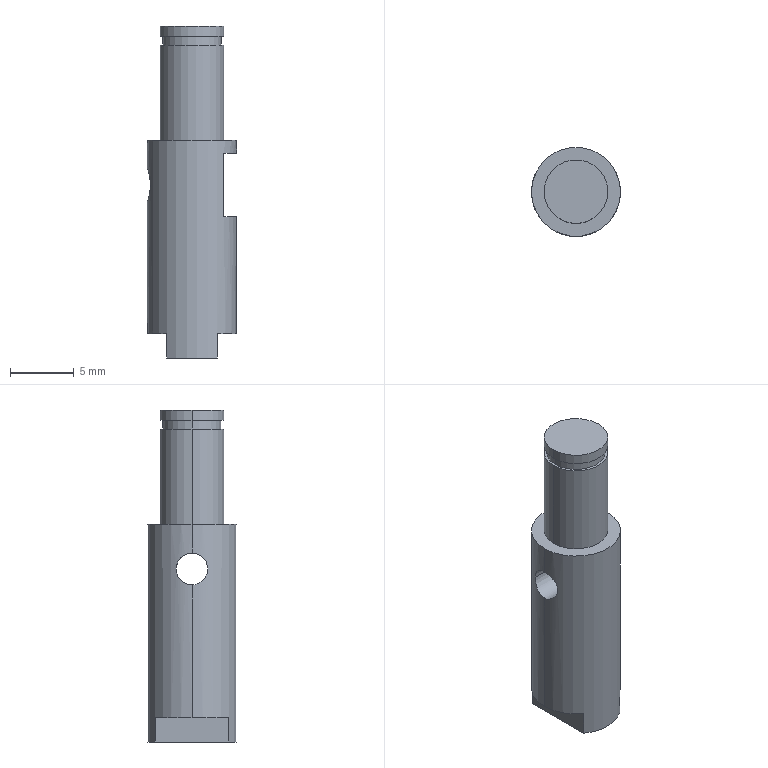Part | NX | 1 solid | 30 faces | box 7 x 7 x 26.1 mm | volume 718.496 mm3 | plane 12 | cylinder 12 | cone 6 | commonest cylinder face diameters 2.5 x4 5 x4 4.6 x2 7 x2
STEP:
#1=CARTESIAN_POINT('',(-2.5,0.,9.));
#2=VERTEX_POINT('',#1);
#3=CARTESIAN_POINT('',(2.5,0.,9.));
#4=VERTEX_POINT('',#3);
#5=CARTESIAN_POINT('',(0.,0.,9.));
#6=DIRECTION('',(0.,0.,-1.));
#7=DIRECTION('',(1.,0.,0.));
#8=AXIS2_PLACEMENT_3D('',#5,#6,#7);
#9=CIRCLE('',#8,2.5);
#10=EDGE_CURVE('',#2,#4,#9,.T.);
#11=ORIENTED_EDGE('',*,*,#10,.F.);
#12=CARTESIAN_POINT('',(0.,0.,9.));
#13=DIRECTION('',(0.,0.,-1.));
#14=DIRECTION('',(1.,0.,0.));
#15=AXIS2_PLACEMENT_3D('',#12,#13,#14);
#16=CIRCLE('',#15,2.5);
#17=EDGE_CURVE('',#4,#2,#16,.T.);
#18=ORIENTED_EDGE('',*,*,#17,.F.);
#19=EDGE_LOOP('',(#11,#18));
#20=FACE_BOUND('',#19,.T.);
#21=CARTESIAN_POINT('',(0.,0.,9.));
#22=DIRECTION('',(0.,0.,1.));
#23=DIRECTION('',(1.,0.,0.));
#24=AXIS2_PLACEMENT_3D('',#21,#22,#23);
#25=PLANE('',#24);
#26=ADVANCED_FACE('',(#20),#25,.T.);
#27=ORIENTED_EDGE('',*,*,#10,.T.);
#28=CARTESIAN_POINT('',(2.5,0.,8.2));
#29=VERTEX_POINT('',#28);
#30=CARTESIAN_POINT('',(2.5,0.,0.));
#31=DIRECTION('',(0.,0.,1.));
#32=VECTOR('',#31,1000.);
#33=LINE('',#30,#32);
#34=EDGE_CURVE('',#29,#4,#33,.T.);
#35=ORIENTED_EDGE('',*,*,#34,.F.);
#36=CARTESIAN_POINT('',(-2.5,0.,8.2));
#37=VERTEX_POINT('',#36);
#38=CARTESIAN_POINT('',(0.,0.,8.2));
#39=DIRECTION('',(0.,0.,1.));
#40=DIRECTION('',(-1.,0.,0.));
#41=AXIS2_PLACEMENT_3D('',#38,#39,#40);
#42=CIRCLE('',#41,2.5);
#43=EDGE_CURVE('',#29,#37,#42,.T.);
#44=ORIENTED_EDGE('',*,*,#43,.T.);
#45=CARTESIAN_POINT('',(-2.5,0.,0.));
#46=DIRECTION('',(0.,0.,1.));
#47=VECTOR('',#46,1000.);
#48=LINE('',#45,#47);
#49=EDGE_CURVE('',#37,#2,#48,.T.);
#50=ORIENTED_EDGE('',*,*,#49,.T.);
#51=EDGE_LOOP('',(#27,#35,#44,#50));
#52=FACE_BOUND('',#51,.T.);
#53=CARTESIAN_POINT('',(0.,0.,0.));
#54=DIRECTION('',(0.,0.,1.));
#55=DIRECTION('',(1.,0.,0.));
#56=AXIS2_PLACEMENT_3D('',#53,#54,#55);
#57=CYLINDRICAL_SURFACE('',#56,2.5);
#58=ADVANCED_FACE('',(#52),#57,.T.);
#59=ORIENTED_EDGE('',*,*,#43,.F.);
#60=CARTESIAN_POINT('',(0.,0.,8.2));
#61=DIRECTION('',(0.,0.,1.));
#62=DIRECTION('',(-1.,0.,0.));
#63=AXIS2_PLACEMENT_3D('',#60,#61,#62);
#64=CIRCLE('',#63,2.5);
#65=EDGE_CURVE('',#37,#29,#64,.T.);
#66=ORIENTED_EDGE('',*,*,#65,.F.);
#67=EDGE_LOOP('',(#59,#66));
#68=FACE_BOUND('',#67,.T.);
#69=CARTESIAN_POINT('',(2.3,0.,8.2));
#70=VERTEX_POINT('',#69);
#71=CARTESIAN_POINT('',(-2.3,0.,8.2));
#72=VERTEX_POINT('',#71);
#73=CARTESIAN_POINT('',(0.,0.,8.2));
#74=DIRECTION('',(0.,0.,-1.));
#75=DIRECTION('',(1.,0.,0.));
#76=AXIS2_PLACEMENT_3D('',#73,#74,#75);
#77=CIRCLE('',#76,2.3);
#78=EDGE_CURVE('',#70,#72,#77,.T.);
#79=ORIENTED_EDGE('',*,*,#78,.F.);
#80=CARTESIAN_POINT('',(0.,0.,8.2));
#81=DIRECTION('',(0.,0.,-1.));
#82=DIRECTION('',(1.,0.,0.));
#83=AXIS2_PLACEMENT_3D('',#80,#81,#82);
#84=CIRCLE('',#83,2.3);
#85=EDGE_CURVE('',#72,#70,#84,.T.);
#86=ORIENTED_EDGE('',*,*,#85,.F.);
#87=EDGE_LOOP('',(#79,#86));
#88=FACE_BOUND('',#87,.T.);
#89=CARTESIAN_POINT('',(0.,0.,8.2));
#90=DIRECTION('',(0.,0.,-1.));
#91=DIRECTION('',(0.,-1.,0.));
#92=AXIS2_PLACEMENT_3D('',#89,#90,#91);
#93=PLANE('',#92);
#94=ADVANCED_FACE('',(#68,#88),#93,.T.);
#95=CARTESIAN_POINT('',(-2.,2.872,-17.1));
#96=VERTEX_POINT('',#95);
#97=CARTESIAN_POINT('',(2.,2.872,-17.1));
#98=VERTEX_POINT('',#97);
#99=CARTESIAN_POINT('',(0.,0.,-17.1));
#100=DIRECTION('',(0.,0.,-1.));
#101=DIRECTION('',(-1.,0.,0.));
#102=AXIS2_PLACEMENT_3D('',#99,#100,#101);
#103=CIRCLE('',#102,3.5);
#104=EDGE_CURVE('',#96,#98,#103,.T.);
#105=ORIENTED_EDGE('',*,*,#104,.T.);
#106=CARTESIAN_POINT('',(2.,-2.872,-17.1));
#107=VERTEX_POINT('',#106);
#108=CARTESIAN_POINT('',(2.,0.,-17.1));
#109=DIRECTION('',(0.,-1.,0.));
#110=VECTOR('',#109,1000.);
#111=LINE('',#108,#110);
#112=EDGE_CURVE('',#98,#107,#111,.T.);
#113=ORIENTED_EDGE('',*,*,#112,.T.);
#114=CARTESIAN_POINT('',(-2.,-2.872,-17.1));
#115=VERTEX_POINT('',#114);
#116=CARTESIAN_POINT('',(0.,0.,-17.1));
#117=DIRECTION('',(0.,0.,-1.));
#118=DIRECTION('',(-1.,0.,0.));
#119=AXIS2_PLACEMENT_3D('',#116,#117,#118);
#120=CIRCLE('',#119,3.5);
#121=EDGE_CURVE('',#107,#115,#120,.T.);
#122=ORIENTED_EDGE('',*,*,#121,.T.);
#123=CARTESIAN_POINT('',(-2.,0.,-17.1));
#124=DIRECTION('',(0.,-1.,0.));
#125=VECTOR('',#124,1000.);
#126=LINE('',#123,#125);
#127=EDGE_CURVE('',#96,#115,#126,.T.);
#128=ORIENTED_EDGE('',*,*,#127,.F.);
#129=EDGE_LOOP('',(#105,#113,#122,#128));
#130=FACE_BOUND('',#129,.T.);
#131=CARTESIAN_POINT('',(1.7,0.,-17.1));
#132=VERTEX_POINT('',#131);
#133=CARTESIAN_POINT('',(-1.7,0.,-17.1));
#134=VERTEX_POINT('',#133);
#135=CARTESIAN_POINT('',(0.,0.,-17.1));
#136=DIRECTION('',(0.,0.,-1.));
#137=DIRECTION('',(-1.,0.,0.));
#138=AXIS2_PLACEMENT_3D('',#135,#136,#137);
#139=CIRCLE('',#138,1.7);
#140=EDGE_CURVE('',#132,#134,#139,.T.);
#141=ORIENTED_EDGE('',*,*,#140,.F.);
#142=CARTESIAN_POINT('',(0.,0.,-17.1));
#143=DIRECTION('',(0.,0.,-1.));
#144=DIRECTION('',(-1.,0.,0.));
#145=AXIS2_PLACEMENT_3D('',#142,#143,#144);
#146=CIRCLE('',#145,1.7);
#147=EDGE_CURVE('',#134,#132,#146,.T.);
#148=ORIENTED_EDGE('',*,*,#147,.F.);
#149=EDGE_LOOP('',(#141,#148));
#150=FACE_BOUND('',#149,.T.);
#151=CARTESIAN_POINT('',(0.,0.,-17.1));
#152=DIRECTION('',(0.,0.,-1.));
#153=DIRECTION('',(0.,-1.,0.));
#154=AXIS2_PLACEMENT_3D('',#151,#152,#153);
#155=PLANE('',#154);
#156=ADVANCED_FACE('',(#130,#150),#155,.T.);
#157=ORIENTED_EDGE('',*,*,#78,.T.);
#158=CARTESIAN_POINT('',(-2.3,0.,7.5));
#159=VERTEX_POINT('',#158);
#160=CARTESIAN_POINT('',(-2.3,0.,8.235));
#161=DIRECTION('',(0.,0.,-1.));
#162=VECTOR('',#161,1000.);
#163=LINE('',#160,#162);
#164=EDGE_CURVE('',#159,#72,#163,.F.);
#165=ORIENTED_EDGE('',*,*,#164,.F.);
#166=CARTESIAN_POINT('',(2.3,0.,7.5));
#167=VERTEX_POINT('',#166);
#168=CARTESIAN_POINT('',(0.,0.,7.5));
#169=DIRECTION('',(0.,0.,1.));
#170=DIRECTION('',(1.,0.,0.));
#171=AXIS2_PLACEMENT_3D('',#168,#169,#170);
#172=CIRCLE('',#171,2.3);
#173=EDGE_CURVE('',#159,#167,#172,.T.);
#174=ORIENTED_EDGE('',*,*,#173,.T.);
#175=CARTESIAN_POINT('',(2.3,0.,8.235));
#176=DIRECTION('',(0.,0.,-1.));
#177=VECTOR('',#176,1000.);
#178=LINE('',#175,#177);
#179=EDGE_CURVE('',#167,#70,#178,.F.);
#180=ORIENTED_EDGE('',*,*,#179,.T.);
#181=EDGE_LOOP('',(#157,#165,#174,#180));
#182=FACE_BOUND('',#181,.T.);
#183=CARTESIAN_POINT('',(0.,0.,8.235));
#184=DIRECTION('',(0.,0.,-1.));
#185=DIRECTION('',(-1.,0.,0.));
#186=AXIS2_PLACEMENT_3D('',#183,#184,#185);
#187=CYLINDRICAL_SURFACE('',#186,2.3);
#188=ADVANCED_FACE('',(#182),#187,.T.);
#189=CARTESIAN_POINT('',(-3.269,1.25,-3.5));
#190=VERTEX_POINT('',#189);
#191=CARTESIAN_POINT('',(-3.5,0.,-2.25));
#192=VERTEX_POINT('',#191);
#193=CARTESIAN_POINT('',(-3.5,0.,-2.25));
#194=CARTESIAN_POINT('',(-3.5,0.1562,-2.25));
#195=CARTESIAN_POINT('',(-3.476,0.4429,-2.317));
#196=CARTESIAN_POINT('',(-3.44,0.6524,-2.427));
#197=CARTESIAN_POINT('',(-3.387,0.8925,-2.603));
#198=CARTESIAN_POINT('',(-3.33,1.082,-2.861));
#199=CARTESIAN_POINT('',(-3.296,1.178,-3.049));
#200=CARTESIAN_POINT('',(-3.269,1.25,-3.345));
#201=CARTESIAN_POINT('',(-3.269,1.25,-3.5));
#202=B_SPLINE_CURVE_WITH_KNOTS('',3,(#193,#194,#195,#196,#197,#198,#199,#200,#201),.UNSPECIFIED.,.F.,.F.,(4,1,1,1,1,1,4),(0.,0.25,0.375,0.5,0.625,0.75,1.),.UNSPECIFIED.);
#203=EDGE_CURVE('',#190,#192,#202,.F.);
#204=ORIENTED_EDGE('',*,*,#203,.F.);
#205=CARTESIAN_POINT('',(2.24,1.25,-3.5));
#206=VERTEX_POINT('',#205);
#207=CARTESIAN_POINT('',(2.5,1.25,-3.5));
#208=DIRECTION('',(1.,0.,0.));
#209=VECTOR('',#208,1000.);
#210=LINE('',#207,#209);
#211=EDGE_CURVE('',#190,#206,#210,.T.);
#212=ORIENTED_EDGE('',*,*,#211,.T.);
#213=CARTESIAN_POINT('',(2.24,-1.25,-3.5));
#214=VERTEX_POINT('',#213);
#215=CARTESIAN_POINT('',(2.24,0.,-3.5));
#216=DIRECTION('',(1.,0.,0.));
#217=DIRECTION('',(0.,-1.,0.));
#218=AXIS2_PLACEMENT_3D('',#215,#216,#217);
#219=CIRCLE('',#218,1.25);
#220=EDGE_CURVE('',#206,#214,#219,.T.);
#221=ORIENTED_EDGE('',*,*,#220,.T.);
#222=CARTESIAN_POINT('',(-3.269,-1.25,-3.5));
#223=VERTEX_POINT('',#222);
#224=CARTESIAN_POINT('',(2.5,-1.25,-3.5));
#225=DIRECTION('',(1.,0.,0.));
#226=VECTOR('',#225,1000.);
#227=LINE('',#224,#226);
#228=EDGE_CURVE('',#223,#214,#227,.T.);
#229=ORIENTED_EDGE('',*,*,#228,.F.);
#230=CARTESIAN_POINT('',(-3.269,-1.25,-3.5));
#231=CARTESIAN_POINT('',(-3.269,-1.25,-3.345));
#232=CARTESIAN_POINT('',(-3.296,-1.178,-3.049));
#233=CARTESIAN_POINT('',(-3.33,-1.082,-2.86));
#234=CARTESIAN_POINT('',(-3.387,-0.8925,-2.603));
#235=CARTESIAN_POINT('',(-3.44,-0.6525,-2.427));
#236=CARTESIAN_POINT('',(-3.476,-0.4428,-2.317));
#237=CARTESIAN_POINT('',(-3.5,-0.1562,-2.25));
#238=CARTESIAN_POINT('',(-3.5,0.,-2.25));
#239=B_SPLINE_CURVE_WITH_KNOTS('',3,(#230,#231,#232,#233,#234,#235,#236,#237,#238),.UNSPECIFIED.,.F.,.F.,(4,1,1,1,1,1,4),(0.,0.25,0.375,0.5,0.625,0.75,1.),.UNSPECIFIED.);
#240=EDGE_CURVE('',#192,#223,#239,.F.);
#241=ORIENTED_EDGE('',*,*,#240,.F.);
#242=EDGE_LOOP('',(#204,#212,#221,#229,#241));
#243=FACE_BOUND('',#242,.T.);
#244=CARTESIAN_POINT('',(2.5,0.,-3.5));
#245=DIRECTION('',(1.,0.,0.));
#246=DIRECTION('',(0.,-1.,0.));
#247=AXIS2_PLACEMENT_3D('',#244,#245,#246);
#248=CYLINDRICAL_SURFACE('',#247,1.25);
#249=ADVANCED_FACE('',(#243),#248,.F.);
#250=CARTESIAN_POINT('',(2.5,0.,7.5));
#251=VERTEX_POINT('',#250);
#252=CARTESIAN_POINT('',(-2.5,0.,7.5));
#253=VERTEX_POINT('',#252);
#254=CARTESIAN_POINT('',(0.,0.,7.5));
#255=DIRECTION('',(0.,0.,-1.));
#256=DIRECTION('',(1.,0.,0.));
#257=AXIS2_PLACEMENT_3D('',#254,#255,#256);
#258=CIRCLE('',#257,2.5);
#259=EDGE_CURVE('',#251,#253,#258,.T.);
#260=ORIENTED_EDGE('',*,*,#259,.F.);
#261=CARTESIAN_POINT('',(0.,0.,7.5));
#262=DIRECTION('',(0.,0.,-1.));
#263=DIRECTION('',(1.,0.,0.));
#264=AXIS2_PLACEMENT_3D('',#261,#262,#263);
#265=CIRCLE('',#264,2.5);
#266=EDGE_CURVE('',#253,#251,#265,.T.);
#267=ORIENTED_EDGE('',*,*,#266,.F.);
#268=EDGE_LOOP('',(#260,#267));
#269=FACE_BOUND('',#268,.T.);
#270=ORIENTED_EDGE('',*,*,#173,.F.);
#271=CARTESIAN_POINT('',(0.,0.,7.5));
#272=DIRECTION('',(0.,0.,1.));
#273=DIRECTION('',(1.,0.,0.));
#274=AXIS2_PLACEMENT_3D('',#271,#272,#273);
#275=CIRCLE('',#274,2.3);
#276=EDGE_CURVE('',#167,#159,#275,.T.);
#277=ORIENTED_EDGE('',*,*,#276,.F.);
#278=EDGE_LOOP('',(#270,#277));
#279=FACE_BOUND('',#278,.T.);
#280=CARTESIAN_POINT('',(0.,0.,7.5));
#281=DIRECTION('',(0.,0.,-1.));
#282=DIRECTION('',(0.,-1.,0.));
#283=AXIS2_PLACEMENT_3D('',#280,#281,#282);
#284=PLANE('',#283);
#285=ADVANCED_FACE('',(#269,#279),#284,.F.);
#286=ORIENTED_EDGE('',*,*,#259,.T.);
#287=CARTESIAN_POINT('',(-2.5,0.,0.));
#288=VERTEX_POINT('',#287);
#289=CARTESIAN_POINT('',(-2.5,0.,0.));
#290=DIRECTION('',(0.,0.,1.));
#291=VECTOR('',#290,1000.);
#292=LINE('',#289,#291);
#293=EDGE_CURVE('',#253,#288,#292,.F.);
#294=ORIENTED_EDGE('',*,*,#293,.T.);
#295=CARTESIAN_POINT('',(2.5,0.,0.));
#296=VERTEX_POINT('',#295);
#297=CARTESIAN_POINT('',(0.,0.,0.));
#298=DIRECTION('',(0.,0.,1.));
#299=DIRECTION('',(1.,0.,0.));
#300=AXIS2_PLACEMENT_3D('',#297,#298,#299);
#301=CIRCLE('',#300,2.5);
#302=EDGE_CURVE('',#288,#296,#301,.T.);
#303=ORIENTED_EDGE('',*,*,#302,.T.);
#304=CARTESIAN_POINT('',(2.5,0.,0.));
#305=DIRECTION('',(0.,0.,1.));
#306=VECTOR('',#305,1000.);
#307=LINE('',#304,#306);
#308=EDGE_CURVE('',#251,#296,#307,.F.);
#309=ORIENTED_EDGE('',*,*,#308,.F.);
#310=EDGE_LOOP('',(#286,#294,#303,#309));
#311=FACE_BOUND('',#310,.T.);
#312=CARTESIAN_POINT('',(0.,0.,0.));
#313=DIRECTION('',(0.,0.,1.));
#314=DIRECTION('',(1.,0.,0.));
#315=AXIS2_PLACEMENT_3D('',#312,#313,#314);
#316=CYLINDRICAL_SURFACE('',#315,2.5);
#317=ADVANCED_FACE('',(#311),#316,.T.);
#318=CARTESIAN_POINT('',(2.24,0.,-3.5));
#319=DIRECTION('',(1.,0.,0.));
#320=DIRECTION('',(0.,-1.,0.));
#321=AXIS2_PLACEMENT_3D('',#318,#319,#320);
#322=CIRCLE('',#321,1.25);
#323=EDGE_CURVE('',#214,#206,#322,.T.);
#324=ORIENTED_EDGE('',*,*,#323,.F.);
#325=CARTESIAN_POINT('',(2.5,-1.7,-3.5));
#326=VERTEX_POINT('',#325);
#327=CARTESIAN_POINT('',(2.24,-1.25,-3.5));
#328=DIRECTION('',(0.5,-0.866,0.));
#329=VECTOR('',#328,1000.);
#330=LINE('',#327,#329);
#331=EDGE_CURVE('',#326,#214,#330,.F.);
#332=ORIENTED_EDGE('',*,*,#331,.F.);
#333=CARTESIAN_POINT('',(2.5,1.7,-3.5));
#334=VERTEX_POINT('',#333);
#335=CARTESIAN_POINT('',(2.5,0.,-3.5));
#336=DIRECTION('',(1.,0.,0.));
#337=DIRECTION('',(0.,-1.,0.));
#338=AXIS2_PLACEMENT_3D('',#335,#336,#337);
#339=CIRCLE('',#338,1.7);
#340=EDGE_CURVE('',#326,#334,#339,.T.);
#341=ORIENTED_EDGE('',*,*,#340,.T.);
#342=CARTESIAN_POINT('',(2.24,1.25,-3.5));
#343=DIRECTION('',(0.5,0.866,0.));
#344=VECTOR('',#343,1000.);
#345=LINE('',#342,#344);
#346=EDGE_CURVE('',#334,#206,#345,.F.);
#347=ORIENTED_EDGE('',*,*,#346,.T.);
#348=EDGE_LOOP('',(#324,#332,#341,#347));
#349=FACE_BOUND('',#348,.T.);
#350=CARTESIAN_POINT('',(2.24,0.,-3.5));
#351=DIRECTION('',(1.,0.,0.));
#352=DIRECTION('',(0.,-1.,0.));
#353=AXIS2_PLACEMENT_3D('',#350,#351,#352);
#354=CONICAL_SURFACE('',#353,1.25,1.047);
#355=ADVANCED_FACE('',(#349),#354,.F.);
#356=CARTESIAN_POINT('',(2.5,2.449,-1.));
#357=VERTEX_POINT('',#356);
#358=CARTESIAN_POINT('',(2.5,2.449,-6.));
#359=VERTEX_POINT('',#358);
#360=CARTESIAN_POINT('',(2.5,2.449,0.));
#361=DIRECTION('',(0.,0.,-1.));
#362=VECTOR('',#361,1000.);
#363=LINE('',#360,#362);
#364=EDGE_CURVE('',#357,#359,#363,.T.);
#365=ORIENTED_EDGE('',*,*,#364,.F.);
#366=CARTESIAN_POINT('',(2.5,-2.449,-1.));
#367=VERTEX_POINT('',#366);
#368=CARTESIAN_POINT('',(2.5,0.,-1.));
#369=DIRECTION('',(0.,-1.,0.));
#370=VECTOR('',#369,1000.);
#371=LINE('',#368,#370);
#372=EDGE_CURVE('',#357,#367,#371,.T.);
#373=ORIENTED_EDGE('',*,*,#372,.T.);
#374=CARTESIAN_POINT('',(2.5,-2.449,-6.));
#375=VERTEX_POINT('',#374);
#376=CARTESIAN_POINT('',(2.5,-2.449,0.));
#377=DIRECTION('',(0.,0.,-1.));
#378=VECTOR('',#377,1000.);
#379=LINE('',#376,#378);
#380=EDGE_CURVE('',#367,#375,#379,.T.);
#381=ORIENTED_EDGE('',*,*,#380,.T.);
#382=CARTESIAN_POINT('',(2.5,0.,-6.));
#383=DIRECTION('',(0.,1.,0.));
#384=VECTOR('',#383,1000.);
#385=LINE('',#382,#384);
#386=EDGE_CURVE('',#375,#359,#385,.T.);
#387=ORIENTED_EDGE('',*,*,#386,.T.);
#388=EDGE_LOOP('',(#365,#373,#381,#387));
#389=FACE_BOUND('',#388,.T.);
#390=ORIENTED_EDGE('',*,*,#340,.F.);
#391=CARTESIAN_POINT('',(2.5,0.,-3.5));
#392=DIRECTION('',(1.,0.,0.));
#393=DIRECTION('',(0.,-1.,0.));
#394=AXIS2_PLACEMENT_3D('',#391,#392,#393);
#395=CIRCLE('',#394,1.7);
#396=EDGE_CURVE('',#334,#326,#395,.T.);
#397=ORIENTED_EDGE('',*,*,#396,.F.);
#398=EDGE_LOOP('',(#390,#397));
#399=FACE_BOUND('',#398,.T.);
#400=CARTESIAN_POINT('',(2.5,3.5,-6.));
#401=DIRECTION('',(-1.,0.,0.));
#402=DIRECTION('',(0.,0.,1.));
#403=AXIS2_PLACEMENT_3D('',#400,#401,#402);
#404=PLANE('',#403);
#405=ADVANCED_FACE('',(#389,#399),#404,.F.);
#406=CARTESIAN_POINT('',(3.5,0.,-15.2));
#407=VERTEX_POINT('',#406);
#408=CARTESIAN_POINT('',(2.,-2.872,-15.2));
#409=VERTEX_POINT('',#408);
#410=CARTESIAN_POINT('',(0.,0.,-15.2));
#411=DIRECTION('',(0.,0.,-1.));
#412=DIRECTION('',(-1.,0.,0.));
#413=AXIS2_PLACEMENT_3D('',#410,#411,#412);
#414=CIRCLE('',#413,3.5);
#415=EDGE_CURVE('',#407,#409,#414,.T.);
#416=ORIENTED_EDGE('',*,*,#415,.F.);
#417=CARTESIAN_POINT('',(3.5,0.,-6.));
#418=VERTEX_POINT('',#417);
#419=CARTESIAN_POINT('',(3.5,0.,0.));
#420=DIRECTION('',(0.,0.,-1.));
#421=VECTOR('',#420,1000.);
#422=LINE('',#419,#421);
#423=EDGE_CURVE('',#418,#407,#422,.T.);
#424=ORIENTED_EDGE('',*,*,#423,.F.);
#425=CARTESIAN_POINT('',(0.,0.,-6.));
#426=DIRECTION('',(0.,0.,-1.));
#427=DIRECTION('',(-1.,0.,0.));
#428=AXIS2_PLACEMENT_3D('',#425,#426,#427);
#429=CIRCLE('',#428,3.5);
#430=EDGE_CURVE('',#418,#375,#429,.T.);
#431=ORIENTED_EDGE('',*,*,#430,.T.);
#432=ORIENTED_EDGE('',*,*,#380,.F.);
#433=CARTESIAN_POINT('',(3.5,0.,-1.));
#434=VERTEX_POINT('',#433);
#435=CARTESIAN_POINT('',(0.,0.,-1.));
#436=DIRECTION('',(0.,0.,-1.));
#437=DIRECTION('',(-1.,0.,0.));
#438=AXIS2_PLACEMENT_3D('',#435,#436,#437);
#439=CIRCLE('',#438,3.5);
#440=EDGE_CURVE('',#434,#367,#439,.T.);
#441=ORIENTED_EDGE('',*,*,#440,.F.);
#442=CARTESIAN_POINT('',(3.5,0.,0.));
#443=VERTEX_POINT('',#442);
#444=CARTESIAN_POINT('',(3.5,0.,0.));
#445=DIRECTION('',(0.,0.,-1.));
#446=VECTOR('',#445,1000.);
#447=LINE('',#444,#446);
#448=EDGE_CURVE('',#434,#443,#447,.F.);
#449=ORIENTED_EDGE('',*,*,#448,.T.);
#450=CARTESIAN_POINT('',(-3.5,0.,0.));
#451=VERTEX_POINT('',#450);
#452=CARTESIAN_POINT('',(0.,0.,0.));
#453=DIRECTION('',(0.,0.,-1.));
#454=DIRECTION('',(-1.,0.,0.));
#455=AXIS2_PLACEMENT_3D('',#452,#453,#454);
#456=CIRCLE('',#455,3.5);
#457=EDGE_CURVE('',#443,#451,#456,.T.);
#458=ORIENTED_EDGE('',*,*,#457,.T.);
#459=CARTESIAN_POINT('',(-3.5,0.,0.));
#460=DIRECTION('',(0.,0.,-1.));
#461=VECTOR('',#460,1000.);
#462=LINE('',#459,#461);
#463=EDGE_CURVE('',#192,#451,#462,.F.);
#464=ORIENTED_EDGE('',*,*,#463,.F.);
#465=ORIENTED_EDGE('',*,*,#240,.T.);
#466=CARTESIAN_POINT('',(-3.5,0.,-4.75));
#467=VERTEX_POINT('',#466);
#468=CARTESIAN_POINT('',(-3.269,-1.25,-3.5));
#469=CARTESIAN_POINT('',(-3.269,-1.249,-4.165));
#470=CARTESIAN_POINT('',(-3.5,-0.6651,-4.75));
#471=CARTESIAN_POINT('',(-3.5,0.,-4.75));
#472=B_SPLINE_CURVE_WITH_KNOTS('',3,(#468,#469,#470,#471),.UNSPECIFIED.,.F.,.F.,(4,4),(0.,1.),.UNSPECIFIED.);
#473=EDGE_CURVE('',#223,#467,#472,.T.);
#474=ORIENTED_EDGE('',*,*,#473,.T.);
#475=CARTESIAN_POINT('',(-3.5,0.,-15.2));
#476=VERTEX_POINT('',#475);
#477=CARTESIAN_POINT('',(-3.5,0.,0.));
#478=DIRECTION('',(0.,0.,-1.));
#479=VECTOR('',#478,1000.);
#480=LINE('',#477,#479);
#481=EDGE_CURVE('',#467,#476,#480,.T.);
#482=ORIENTED_EDGE('',*,*,#481,.T.);
#483=CARTESIAN_POINT('',(-2.,-2.872,-15.2));
#484=VERTEX_POINT('',#483);
#485=CARTESIAN_POINT('',(0.,0.,-15.2));
#486=DIRECTION('',(0.,0.,-1.));
#487=DIRECTION('',(-1.,0.,0.));
#488=AXIS2_PLACEMENT_3D('',#485,#486,#487);
#489=CIRCLE('',#488,3.5);
#490=EDGE_CURVE('',#484,#476,#489,.T.);
#491=ORIENTED_EDGE('',*,*,#490,.F.);
#492=CARTESIAN_POINT('',(-2.,-2.872,0.));
#493=DIRECTION('',(0.,0.,-1.));
#494=VECTOR('',#493,1000.);
#495=LINE('',#492,#494);
#496=EDGE_CURVE('',#484,#115,#495,.T.);
#497=ORIENTED_EDGE('',*,*,#496,.T.);
#498=ORIENTED_EDGE('',*,*,#121,.F.);
#499=CARTESIAN_POINT('',(2.,-2.872,0.));
#500=DIRECTION('',(0.,0.,-1.));
#501=VECTOR('',#500,1000.);
#502=LINE('',#499,#501);
#503=EDGE_CURVE('',#409,#107,#502,.T.);
#504=ORIENTED_EDGE('',*,*,#503,.F.);
#505=EDGE_LOOP('',(#416,#424,#431,#432,#441,#449,#458,#464,#465,#474,#482,#491,#497,#498,#504));
#506=FACE_BOUND('',#505,.T.);
#507=CARTESIAN_POINT('',(0.,0.,0.));
#508=DIRECTION('',(0.,0.,-1.));
#509=DIRECTION('',(-1.,0.,0.));
#510=AXIS2_PLACEMENT_3D('',#507,#508,#509);
#511=CYLINDRICAL_SURFACE('',#510,3.5);
#512=ADVANCED_FACE('',(#506),#511,.T.);
#513=CARTESIAN_POINT('',(0.,0.,-7.599));
#514=VERTEX_POINT('',#513);
#515=CARTESIAN_POINT('',(1.25,0.,-8.35));
#516=VERTEX_POINT('',#515);
#517=CARTESIAN_POINT('',(1.25,0.,-8.35));
#518=DIRECTION('',(0.8572,0.,-0.515));
#519=VECTOR('',#518,1000.);
#520=LINE('',#517,#519);
#521=EDGE_CURVE('',#514,#516,#520,.T.);
#522=ORIENTED_EDGE('',*,*,#521,.T.);
#523=CARTESIAN_POINT('',(-1.25,0.,-8.35));
#524=VERTEX_POINT('',#523);
#525=CARTESIAN_POINT('',(0.,0.,-8.35));
#526=DIRECTION('',(0.,0.,-1.));
#527=DIRECTION('',(-1.,0.,0.));
#528=AXIS2_PLACEMENT_3D('',#525,#526,#527);
#529=CIRCLE('',#528,1.25);
#530=EDGE_CURVE('',#516,#524,#529,.T.);
#531=ORIENTED_EDGE('',*,*,#530,.T.);
#532=CARTESIAN_POINT('',(-1.25,0.,-8.35));
#533=DIRECTION('',(-0.8572,0.,-0.515));
#534=VECTOR('',#533,1000.);
#535=LINE('',#532,#534);
#536=EDGE_CURVE('',#514,#524,#535,.T.);
#537=ORIENTED_EDGE('',*,*,#536,.F.);
#538=EDGE_LOOP('',(#522,#531,#537));
#539=FACE_BOUND('',#538,.T.);
#540=CARTESIAN_POINT('',(0.,0.,-8.35));
#541=DIRECTION('',(0.,0.,-1.));
#542=DIRECTION('',(-1.,0.,0.));
#543=AXIS2_PLACEMENT_3D('',#540,#541,#542);
#544=CONICAL_SURFACE('',#543,1.25,1.03);
#545=ADVANCED_FACE('',(#539),#544,.F.);
#546=CARTESIAN_POINT('',(-2.,2.872,-15.2));
#547=VERTEX_POINT('',#546);
#548=CARTESIAN_POINT('',(0.,0.,-15.2));
#549=DIRECTION('',(0.,0.,-1.));
#550=DIRECTION('',(-1.,0.,0.));
#551=AXIS2_PLACEMENT_3D('',#548,#549,#550);
#552=CIRCLE('',#551,3.5);
#553=EDGE_CURVE('',#476,#547,#552,.T.);
#554=ORIENTED_EDGE('',*,*,#553,.T.);
#555=CARTESIAN_POINT('',(-2.,0.,-15.2));
#556=DIRECTION('',(0.,-1.,0.));
#557=VECTOR('',#556,1000.);
#558=LINE('',#555,#557);
#559=EDGE_CURVE('',#547,#484,#558,.T.);
#560=ORIENTED_EDGE('',*,*,#559,.T.);
#561=ORIENTED_EDGE('',*,*,#490,.T.);
#562=EDGE_LOOP('',(#554,#560,#561));
#563=FACE_BOUND('',#562,.T.);
#564=CARTESIAN_POINT('',(0.,0.,-15.2));
#565=DIRECTION('',(0.,0.,-1.));
#566=DIRECTION('',(0.,-1.,0.));
#567=AXIS2_PLACEMENT_3D('',#564,#565,#566);
#568=PLANE('',#567);
#569=ADVANCED_FACE('',(#563),#568,.T.);
#570=ORIENTED_EDGE('',*,*,#127,.T.);
#571=ORIENTED_EDGE('',*,*,#496,.F.);
#572=ORIENTED_EDGE('',*,*,#559,.F.);
#573=CARTESIAN_POINT('',(-2.,2.872,0.));
#574=DIRECTION('',(0.,0.,-1.));
#575=VECTOR('',#574,1000.);
#576=LINE('',#573,#575);
#577=EDGE_CURVE('',#547,#96,#576,.T.);
#578=ORIENTED_EDGE('',*,*,#577,.T.);
#579=EDGE_LOOP('',(#570,#571,#572,#578));
#580=FACE_BOUND('',#579,.T.);
#581=CARTESIAN_POINT('',(-2.,2.872,-17.35));
#582=DIRECTION('',(1.,0.,0.));
#583=DIRECTION('',(0.,1.,0.));
#584=AXIS2_PLACEMENT_3D('',#581,#582,#583);
#585=PLANE('',#584);
#586=ADVANCED_FACE('',(#580),#585,.F.);
#587=ORIENTED_EDGE('',*,*,#440,.T.);
#588=ORIENTED_EDGE('',*,*,#372,.F.);
#589=CARTESIAN_POINT('',(0.,0.,-1.));
#590=DIRECTION('',(0.,0.,-1.));
#591=DIRECTION('',(-1.,0.,0.));
#592=AXIS2_PLACEMENT_3D('',#589,#590,#591);
#593=CIRCLE('',#592,3.5);
#594=EDGE_CURVE('',#357,#434,#593,.T.);
#595=ORIENTED_EDGE('',*,*,#594,.T.);
#596=EDGE_LOOP('',(#587,#588,#595));
#597=FACE_BOUND('',#596,.T.);
#598=CARTESIAN_POINT('',(2.5,3.5,-1.));
#599=DIRECTION('',(0.,0.,1.));
#600=DIRECTION('',(1.,0.,0.));
#601=AXIS2_PLACEMENT_3D('',#598,#599,#600);
#602=PLANE('',#601);
#603=ADVANCED_FACE('',(#597),#602,.F.);
#604=ORIENTED_EDGE('',*,*,#457,.F.);
#605=CARTESIAN_POINT('',(0.,0.,0.));
#606=DIRECTION('',(0.,0.,-1.));
#607=DIRECTION('',(-1.,0.,0.));
#608=AXIS2_PLACEMENT_3D('',#605,#606,#607);
#609=CIRCLE('',#608,3.5);
#610=EDGE_CURVE('',#451,#443,#609,.T.);
#611=ORIENTED_EDGE('',*,*,#610,.F.);
#612=EDGE_LOOP('',(#604,#611));
#613=FACE_BOUND('',#612,.T.);
#614=CARTESIAN_POINT('',(0.,0.,0.));
#615=DIRECTION('',(0.,0.,1.));
#616=DIRECTION('',(1.,0.,0.));
#617=AXIS2_PLACEMENT_3D('',#614,#615,#616);
#618=CIRCLE('',#617,2.5);
#619=EDGE_CURVE('',#296,#288,#618,.T.);
#620=ORIENTED_EDGE('',*,*,#619,.F.);
#621=ORIENTED_EDGE('',*,*,#302,.F.);
#622=EDGE_LOOP('',(#620,#621));
#623=FACE_BOUND('',#622,.T.);
#624=CARTESIAN_POINT('',(0.,0.,0.));
#625=DIRECTION('',(0.,0.,-1.));
#626=DIRECTION('',(0.,-1.,0.));
#627=AXIS2_PLACEMENT_3D('',#624,#625,#626);
#628=PLANE('',#627);
#629=ADVANCED_FACE('',(#613,#623),#628,.F.);
#630=ORIENTED_EDGE('',*,*,#430,.F.);
#631=CARTESIAN_POINT('',(0.,0.,-6.));
#632=DIRECTION('',(0.,0.,-1.));
#633=DIRECTION('',(-1.,0.,0.));
#634=AXIS2_PLACEMENT_3D('',#631,#632,#633);
#635=CIRCLE('',#634,3.5);
#636=EDGE_CURVE('',#359,#418,#635,.T.);
#637=ORIENTED_EDGE('',*,*,#636,.F.);
#638=ORIENTED_EDGE('',*,*,#386,.F.);
#639=EDGE_LOOP('',(#630,#637,#638));
#640=FACE_BOUND('',#639,.T.);
#641=CARTESIAN_POINT('',(3.7,3.5,-6.));
#642=DIRECTION('',(0.,0.,-1.));
#643=DIRECTION('',(0.,-1.,0.));
#644=AXIS2_PLACEMENT_3D('',#641,#642,#643);
#645=PLANE('',#644);
#646=ADVANCED_FACE('',(#640),#645,.F.);
#647=ORIENTED_EDGE('',*,*,#415,.T.);
#648=CARTESIAN_POINT('',(2.,2.872,-15.2));
#649=VERTEX_POINT('',#648);
#650=CARTESIAN_POINT('',(2.,0.,-15.2));
#651=DIRECTION('',(0.,1.,0.));
#652=VECTOR('',#651,1000.);
#653=LINE('',#650,#652);
#654=EDGE_CURVE('',#409,#649,#653,.T.);
#655=ORIENTED_EDGE('',*,*,#654,.T.);
#656=CARTESIAN_POINT('',(0.,0.,-15.2));
#657=DIRECTION('',(0.,0.,-1.));
#658=DIRECTION('',(-1.,0.,0.));
#659=AXIS2_PLACEMENT_3D('',#656,#657,#658);
#660=CIRCLE('',#659,3.5);
#661=EDGE_CURVE('',#649,#407,#660,.T.);
#662=ORIENTED_EDGE('',*,*,#661,.T.);
#663=EDGE_LOOP('',(#647,#655,#662));
#664=FACE_BOUND('',#663,.T.);
#665=CARTESIAN_POINT('',(0.,0.,-15.2));
#666=DIRECTION('',(0.,0.,-1.));
#667=DIRECTION('',(0.,-1.,0.));
#668=AXIS2_PLACEMENT_3D('',#665,#666,#667);
#669=PLANE('',#668);
#670=ADVANCED_FACE('',(#664),#669,.T.);
#671=CARTESIAN_POINT('',(2.,2.872,0.));
#672=DIRECTION('',(0.,0.,-1.));
#673=VECTOR('',#672,1000.);
#674=LINE('',#671,#673);
#675=EDGE_CURVE('',#649,#98,#674,.T.);
#676=ORIENTED_EDGE('',*,*,#675,.F.);
#677=ORIENTED_EDGE('',*,*,#654,.F.);
#678=ORIENTED_EDGE('',*,*,#503,.T.);
#679=ORIENTED_EDGE('',*,*,#112,.F.);
#680=EDGE_LOOP('',(#676,#677,#678,#679));
#681=FACE_BOUND('',#680,.T.);
#682=CARTESIAN_POINT('',(2.,-2.872,-17.35));
#683=DIRECTION('',(-1.,0.,0.));
#684=DIRECTION('',(0.,0.,1.));
#685=AXIS2_PLACEMENT_3D('',#682,#683,#684);
#686=PLANE('',#685);
#687=ADVANCED_FACE('',(#681),#686,.F.);
#688=CARTESIAN_POINT('',(0.,0.,-8.35));
#689=DIRECTION('',(0.,0.,-1.));
#690=DIRECTION('',(-1.,0.,0.));
#691=AXIS2_PLACEMENT_3D('',#688,#689,#690);
#692=CIRCLE('',#691,1.25);
#693=EDGE_CURVE('',#524,#516,#692,.T.);
#694=ORIENTED_EDGE('',*,*,#693,.F.);
#695=CARTESIAN_POINT('',(-1.25,0.,-16.84));
#696=VERTEX_POINT('',#695);
#697=CARTESIAN_POINT('',(-1.25,0.,-17.35));
#698=DIRECTION('',(0.,0.,-1.));
#699=VECTOR('',#698,1000.);
#700=LINE('',#697,#699);
#701=EDGE_CURVE('',#696,#524,#700,.F.);
#702=ORIENTED_EDGE('',*,*,#701,.F.);
#703=CARTESIAN_POINT('',(1.25,0.,-16.84));
#704=VERTEX_POINT('',#703);
#705=CARTESIAN_POINT('',(0.,0.,-16.84));
#706=DIRECTION('',(0.,0.,-1.));
#707=DIRECTION('',(-1.,0.,0.));
#708=AXIS2_PLACEMENT_3D('',#705,#706,#707);
#709=CIRCLE('',#708,1.25);
#710=EDGE_CURVE('',#696,#704,#709,.T.);
#711=ORIENTED_EDGE('',*,*,#710,.T.);
#712=CARTESIAN_POINT('',(1.25,0.,-17.35));
#713=DIRECTION('',(0.,0.,-1.));
#714=VECTOR('',#713,1000.);
#715=LINE('',#712,#714);
#716=EDGE_CURVE('',#704,#516,#715,.F.);
#717=ORIENTED_EDGE('',*,*,#716,.T.);
#718=EDGE_LOOP('',(#694,#702,#711,#717));
#719=FACE_BOUND('',#718,.T.);
#720=CARTESIAN_POINT('',(0.,0.,-17.35));
#721=DIRECTION('',(0.,0.,-1.));
#722=DIRECTION('',(-1.,0.,0.));
#723=AXIS2_PLACEMENT_3D('',#720,#721,#722);
#724=CYLINDRICAL_SURFACE('',#723,1.25);
#725=ADVANCED_FACE('',(#719),#724,.F.);
#726=ORIENTED_EDGE('',*,*,#140,.T.);
#727=CARTESIAN_POINT('',(-1.25,0.,-16.84));
#728=DIRECTION('',(-0.866,0.,-0.5));
#729=VECTOR('',#728,1000.);
#730=LINE('',#727,#729);
#731=EDGE_CURVE('',#134,#696,#730,.F.);
#732=ORIENTED_EDGE('',*,*,#731,.T.);
#733=CARTESIAN_POINT('',(0.,0.,-16.84));
#734=DIRECTION('',(0.,0.,-1.));
#735=DIRECTION('',(-1.,0.,0.));
#736=AXIS2_PLACEMENT_3D('',#733,#734,#735);
#737=CIRCLE('',#736,1.25);
#738=EDGE_CURVE('',#704,#696,#737,.T.);
#739=ORIENTED_EDGE('',*,*,#738,.F.);
#740=CARTESIAN_POINT('',(1.25,0.,-16.84));
#741=DIRECTION('',(0.866,0.,-0.5));
#742=VECTOR('',#741,1000.);
#743=LINE('',#740,#742);
#744=EDGE_CURVE('',#132,#704,#743,.F.);
#745=ORIENTED_EDGE('',*,*,#744,.F.);
#746=EDGE_LOOP('',(#726,#732,#739,#745));
#747=FACE_BOUND('',#746,.T.);
#748=CARTESIAN_POINT('',(0.,0.,-16.84));
#749=DIRECTION('',(0.,0.,-1.));
#750=DIRECTION('',(-1.,0.,0.));
#751=AXIS2_PLACEMENT_3D('',#748,#749,#750);
#752=CONICAL_SURFACE('',#751,1.25,1.047);
#753=ADVANCED_FACE('',(#747),#752,.F.);
#754=ORIENTED_EDGE('',*,*,#619,.T.);
#755=ORIENTED_EDGE('',*,*,#293,.F.);
#756=ORIENTED_EDGE('',*,*,#266,.T.);
#757=ORIENTED_EDGE('',*,*,#308,.T.);
#758=EDGE_LOOP('',(#754,#755,#756,#757));
#759=FACE_BOUND('',#758,.T.);
#760=CARTESIAN_POINT('',(0.,0.,0.));
#761=DIRECTION('',(0.,0.,1.));
#762=DIRECTION('',(1.,0.,0.));
#763=AXIS2_PLACEMENT_3D('',#760,#761,#762);
#764=CYLINDRICAL_SURFACE('',#763,2.5);
#765=ADVANCED_FACE('',(#759),#764,.T.);
#766=ORIENTED_EDGE('',*,*,#323,.T.);
#767=ORIENTED_EDGE('',*,*,#211,.F.);
#768=CARTESIAN_POINT('',(-3.269,1.25,-3.5));
#769=CARTESIAN_POINT('',(-3.269,1.25,-3.655));
#770=CARTESIAN_POINT('',(-3.296,1.178,-3.951));
#771=CARTESIAN_POINT('',(-3.33,1.082,-4.14));
#772=CARTESIAN_POINT('',(-3.387,0.8925,-4.397));
#773=CARTESIAN_POINT('',(-3.44,0.6525,-4.573));
#774=CARTESIAN_POINT('',(-3.476,0.4428,-4.683));
#775=CARTESIAN_POINT('',(-3.5,0.1563,-4.75));
#776=CARTESIAN_POINT('',(-3.5,0.,-4.75));
#777=B_SPLINE_CURVE_WITH_KNOTS('',3,(#768,#769,#770,#771,#772,#773,#774,#775,#776),.UNSPECIFIED.,.F.,.F.,(4,1,1,1,1,1,4),(0.,0.25,0.375,0.5,0.625,0.75,1.),.UNSPECIFIED.);
#778=EDGE_CURVE('',#467,#190,#777,.F.);
#779=ORIENTED_EDGE('',*,*,#778,.F.);
#780=ORIENTED_EDGE('',*,*,#473,.F.);
#781=ORIENTED_EDGE('',*,*,#228,.T.);
#782=EDGE_LOOP('',(#766,#767,#779,#780,#781));
#783=FACE_BOUND('',#782,.T.);
#784=CARTESIAN_POINT('',(2.5,0.,-3.5));
#785=DIRECTION('',(1.,0.,0.));
#786=DIRECTION('',(0.,-1.,0.));
#787=AXIS2_PLACEMENT_3D('',#784,#785,#786);
#788=CYLINDRICAL_SURFACE('',#787,1.25);
#789=ADVANCED_FACE('',(#783),#788,.F.);
#790=ORIENTED_EDGE('',*,*,#331,.T.);
#791=ORIENTED_EDGE('',*,*,#220,.F.);
#792=ORIENTED_EDGE('',*,*,#346,.F.);
#793=ORIENTED_EDGE('',*,*,#396,.T.);
#794=EDGE_LOOP('',(#790,#791,#792,#793));
#795=FACE_BOUND('',#794,.T.);
#796=CARTESIAN_POINT('',(2.24,0.,-3.5));
#797=DIRECTION('',(1.,0.,0.));
#798=DIRECTION('',(0.,-1.,0.));
#799=AXIS2_PLACEMENT_3D('',#796,#797,#798);
#800=CONICAL_SURFACE('',#799,1.25,1.047);
#801=ADVANCED_FACE('',(#795),#800,.F.);
#802=ORIENTED_EDGE('',*,*,#164,.T.);
#803=ORIENTED_EDGE('',*,*,#85,.T.);
#804=ORIENTED_EDGE('',*,*,#179,.F.);
#805=ORIENTED_EDGE('',*,*,#276,.T.);
#806=EDGE_LOOP('',(#802,#803,#804,#805));
#807=FACE_BOUND('',#806,.T.);
#808=CARTESIAN_POINT('',(0.,0.,8.235));
#809=DIRECTION('',(0.,0.,-1.));
#810=DIRECTION('',(-1.,0.,0.));
#811=AXIS2_PLACEMENT_3D('',#808,#809,#810);
#812=CYLINDRICAL_SURFACE('',#811,2.3);
#813=ADVANCED_FACE('',(#807),#812,.T.);
#814=ORIENTED_EDGE('',*,*,#693,.T.);
#815=ORIENTED_EDGE('',*,*,#521,.F.);
#816=ORIENTED_EDGE('',*,*,#536,.T.);
#817=EDGE_LOOP('',(#814,#815,#816));
#818=FACE_BOUND('',#817,.T.);
#819=CARTESIAN_POINT('',(0.,0.,-8.35));
#820=DIRECTION('',(0.,0.,-1.));
#821=DIRECTION('',(-1.,0.,0.));
#822=AXIS2_PLACEMENT_3D('',#819,#820,#821);
#823=CONICAL_SURFACE('',#822,1.25,1.03);
#824=ADVANCED_FACE('',(#818),#823,.F.);
#825=ORIENTED_EDGE('',*,*,#34,.T.);
#826=ORIENTED_EDGE('',*,*,#17,.T.);
#827=ORIENTED_EDGE('',*,*,#49,.F.);
#828=ORIENTED_EDGE('',*,*,#65,.T.);
#829=EDGE_LOOP('',(#825,#826,#827,#828));
#830=FACE_BOUND('',#829,.T.);
#831=CARTESIAN_POINT('',(0.,0.,0.));
#832=DIRECTION('',(0.,0.,1.));
#833=DIRECTION('',(1.,0.,0.));
#834=AXIS2_PLACEMENT_3D('',#831,#832,#833);
#835=CYLINDRICAL_SURFACE('',#834,2.5);
#836=ADVANCED_FACE('',(#830),#835,.T.);
#837=ORIENTED_EDGE('',*,*,#701,.T.);
#838=ORIENTED_EDGE('',*,*,#530,.F.);
#839=ORIENTED_EDGE('',*,*,#716,.F.);
#840=ORIENTED_EDGE('',*,*,#738,.T.);
#841=EDGE_LOOP('',(#837,#838,#839,#840));
#842=FACE_BOUND('',#841,.T.);
#843=CARTESIAN_POINT('',(0.,0.,-17.35));
#844=DIRECTION('',(0.,0.,-1.));
#845=DIRECTION('',(-1.,0.,0.));
#846=AXIS2_PLACEMENT_3D('',#843,#844,#845);
#847=CYLINDRICAL_SURFACE('',#846,1.25);
#848=ADVANCED_FACE('',(#842),#847,.F.);
#849=ORIENTED_EDGE('',*,*,#463,.T.);
#850=ORIENTED_EDGE('',*,*,#610,.T.);
#851=ORIENTED_EDGE('',*,*,#448,.F.);
#852=ORIENTED_EDGE('',*,*,#594,.F.);
#853=ORIENTED_EDGE('',*,*,#364,.T.);
#854=ORIENTED_EDGE('',*,*,#636,.T.);
#855=ORIENTED_EDGE('',*,*,#423,.T.);
#856=ORIENTED_EDGE('',*,*,#661,.F.);
#857=ORIENTED_EDGE('',*,*,#675,.T.);
#858=ORIENTED_EDGE('',*,*,#104,.F.);
#859=ORIENTED_EDGE('',*,*,#577,.F.);
#860=ORIENTED_EDGE('',*,*,#553,.F.);
#861=ORIENTED_EDGE('',*,*,#481,.F.);
#862=ORIENTED_EDGE('',*,*,#778,.T.);
#863=ORIENTED_EDGE('',*,*,#203,.T.);
#864=EDGE_LOOP('',(#849,#850,#851,#852,#853,#854,#855,#856,#857,#858,#859,#860,#861,#862,#863));
#865=FACE_BOUND('',#864,.T.);
#866=CARTESIAN_POINT('',(0.,0.,0.));
#867=DIRECTION('',(0.,0.,-1.));
#868=DIRECTION('',(-1.,0.,0.));
#869=AXIS2_PLACEMENT_3D('',#866,#867,#868);
#870=CYLINDRICAL_SURFACE('',#869,3.5);
#871=ADVANCED_FACE('',(#865),#870,.T.);
#872=ORIENTED_EDGE('',*,*,#710,.F.);
#873=ORIENTED_EDGE('',*,*,#731,.F.);
#874=ORIENTED_EDGE('',*,*,#147,.T.);
#875=ORIENTED_EDGE('',*,*,#744,.T.);
#876=EDGE_LOOP('',(#872,#873,#874,#875));
#877=FACE_BOUND('',#876,.T.);
#878=CARTESIAN_POINT('',(0.,0.,-16.84));
#879=DIRECTION('',(0.,0.,-1.));
#880=DIRECTION('',(-1.,0.,0.));
#881=AXIS2_PLACEMENT_3D('',#878,#879,#880);
#882=CONICAL_SURFACE('',#881,1.25,1.047);
#883=ADVANCED_FACE('',(#877),#882,.F.);
#884=CLOSED_SHELL('',(#26,#58,#94,#156,#188,#249,#285,#317,#355,#405,#512,#545,#569,#586,#603,#629,#646,#670,#687,#725,#753,#765,#789,#801,#813,#824,#836,#848,#871,#883));
#885=MANIFOLD_SOLID_BREP('',#884);
#886=(LENGTH_UNIT()NAMED_UNIT(*)SI_UNIT(.MILLI.,.METRE.));
#887=UNCERTAINTY_MEASURE_WITH_UNIT(LENGTH_MEASURE(0.0508),#886,'','');
#888=(NAMED_UNIT(*)PLANE_ANGLE_UNIT()SI_UNIT($,.RADIAN.));
#889=(NAMED_UNIT(*)SI_UNIT($,.STERADIAN.)SOLID_ANGLE_UNIT());
#890=(GEOMETRIC_REPRESENTATION_CONTEXT(3)GLOBAL_UNCERTAINTY_ASSIGNED_CONTEXT((#887))GLOBAL_UNIT_ASSIGNED_CONTEXT((#886,#888,#889))REPRESENTATION_CONTEXT('',''));
#891=ADVANCED_BREP_SHAPE_REPRESENTATION('',(#885),#890);